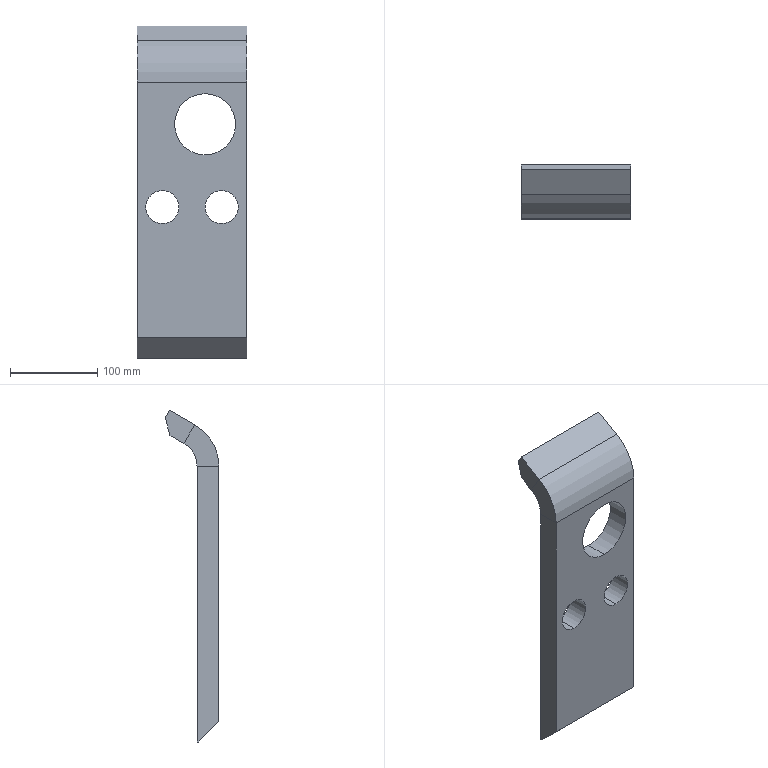Part | SolidWorks | features Chamfer 2, FlatPattern 1, ICE 1, SMBaseFlange 1, SheetMetal 1 | 1 solid | 22 faces | box 126 x 61.5 x 380.651 mm | volume 1041526 mm3 | plane 14 | cylinder 8 | commonest cylinder face diameters 38 x4 70 x2 60 x1 110 x1
STEP:
#1=CARTESIAN_POINT('',(15.,25.,130.));
#2=VERTEX_POINT('',#1);
#3=CARTESIAN_POINT('',(15.,25.,60.));
#4=VERTEX_POINT('',#3);
#5=CARTESIAN_POINT('',(15.,25.,95.));
#6=DIRECTION('',(0.,-1.,0.));
#7=DIRECTION('',(0.,0.,1.));
#8=AXIS2_PLACEMENT_3D('',#5,#6,#7);
#9=CIRCLE('',#8,35.);
#10=EDGE_CURVE('',#2,#4,#9,.T.);
#11=ORIENTED_EDGE('',*,*,#10,.F.);
#12=CARTESIAN_POINT('',(15.,0.,130.));
#13=VERTEX_POINT('',#12);
#14=CARTESIAN_POINT('',(15.,69.,130.));
#15=DIRECTION('',(0.,-1.,0.));
#16=VECTOR('',#15,1000.);
#17=LINE('',#14,#16);
#18=EDGE_CURVE('',#2,#13,#17,.T.);
#19=ORIENTED_EDGE('',*,*,#18,.T.);
#20=CARTESIAN_POINT('',(15.,0.,60.));
#21=VERTEX_POINT('',#20);
#22=CARTESIAN_POINT('',(15.,0.,95.));
#23=DIRECTION('',(0.,1.,0.));
#24=DIRECTION('',(0.,0.,1.));
#25=AXIS2_PLACEMENT_3D('',#22,#23,#24);
#26=CIRCLE('',#25,35.);
#27=EDGE_CURVE('',#21,#13,#26,.T.);
#28=ORIENTED_EDGE('',*,*,#27,.F.);
#29=CARTESIAN_POINT('',(15.,69.,60.));
#30=DIRECTION('',(0.,-1.,0.));
#31=VECTOR('',#30,1000.);
#32=LINE('',#29,#31);
#33=EDGE_CURVE('',#4,#21,#32,.T.);
#34=ORIENTED_EDGE('',*,*,#33,.F.);
#35=EDGE_LOOP('',(#11,#19,#28,#34));
#36=FACE_OUTER_BOUND('',#35,.T.);
#37=CARTESIAN_POINT('',(15.,69.,95.));
#38=DIRECTION('',(0.,-1.,0.));
#39=DIRECTION('',(0.,0.,-1.));
#40=AXIS2_PLACEMENT_3D('',#37,#38,#39);
#41=CYLINDRICAL_SURFACE('',#40,35.);
#42=ADVANCED_FACE('',(#36),#41,.F.);
#43=CARTESIAN_POINT('',(-34.,25.,19.));
#44=VERTEX_POINT('',#43);
#45=CARTESIAN_POINT('',(-34.,25.,-19.));
#46=VERTEX_POINT('',#45);
#47=CARTESIAN_POINT('',(-34.,25.,0.));
#48=DIRECTION('',(0.,-1.,0.));
#49=DIRECTION('',(0.,0.,1.));
#50=AXIS2_PLACEMENT_3D('',#47,#48,#49);
#51=CIRCLE('',#50,19.);
#52=EDGE_CURVE('',#44,#46,#51,.T.);
#53=ORIENTED_EDGE('',*,*,#52,.F.);
#54=CARTESIAN_POINT('',(-34.,0.,19.));
#55=VERTEX_POINT('',#54);
#56=CARTESIAN_POINT('',(-34.,69.,19.));
#57=DIRECTION('',(0.,-1.,0.));
#58=VECTOR('',#57,1000.);
#59=LINE('',#56,#58);
#60=EDGE_CURVE('',#44,#55,#59,.T.);
#61=ORIENTED_EDGE('',*,*,#60,.T.);
#62=CARTESIAN_POINT('',(-34.,0.,-19.));
#63=VERTEX_POINT('',#62);
#64=CARTESIAN_POINT('',(-34.,0.,0.));
#65=DIRECTION('',(0.,1.,0.));
#66=DIRECTION('',(0.,0.,1.));
#67=AXIS2_PLACEMENT_3D('',#64,#65,#66);
#68=CIRCLE('',#67,19.);
#69=EDGE_CURVE('',#63,#55,#68,.T.);
#70=ORIENTED_EDGE('',*,*,#69,.F.);
#71=CARTESIAN_POINT('',(-34.,69.,-19.));
#72=DIRECTION('',(0.,-1.,0.));
#73=VECTOR('',#72,1000.);
#74=LINE('',#71,#73);
#75=EDGE_CURVE('',#46,#63,#74,.T.);
#76=ORIENTED_EDGE('',*,*,#75,.F.);
#77=EDGE_LOOP('',(#53,#61,#70,#76));
#78=FACE_OUTER_BOUND('',#77,.T.);
#79=CARTESIAN_POINT('',(-34.,69.,0.));
#80=DIRECTION('',(0.,-1.,0.));
#81=DIRECTION('',(0.,0.,-1.));
#82=AXIS2_PLACEMENT_3D('',#79,#80,#81);
#83=CYLINDRICAL_SURFACE('',#82,19.);
#84=ADVANCED_FACE('',(#78),#83,.F.);
#85=CARTESIAN_POINT('',(34.,25.,19.));
#86=VERTEX_POINT('',#85);
#87=CARTESIAN_POINT('',(34.,25.,-19.));
#88=VERTEX_POINT('',#87);
#89=CARTESIAN_POINT('',(34.,25.,0.));
#90=DIRECTION('',(0.,-1.,0.));
#91=DIRECTION('',(0.,0.,1.));
#92=AXIS2_PLACEMENT_3D('',#89,#90,#91);
#93=CIRCLE('',#92,19.);
#94=EDGE_CURVE('',#86,#88,#93,.T.);
#95=ORIENTED_EDGE('',*,*,#94,.F.);
#96=CARTESIAN_POINT('',(34.,0.,19.));
#97=VERTEX_POINT('',#96);
#98=CARTESIAN_POINT('',(34.,69.,19.));
#99=DIRECTION('',(0.,-1.,0.));
#100=VECTOR('',#99,1000.);
#101=LINE('',#98,#100);
#102=EDGE_CURVE('',#86,#97,#101,.T.);
#103=ORIENTED_EDGE('',*,*,#102,.T.);
#104=CARTESIAN_POINT('',(34.,0.,-19.));
#105=VERTEX_POINT('',#104);
#106=CARTESIAN_POINT('',(34.,0.,0.));
#107=DIRECTION('',(0.,1.,0.));
#108=DIRECTION('',(0.,0.,1.));
#109=AXIS2_PLACEMENT_3D('',#106,#107,#108);
#110=CIRCLE('',#109,19.);
#111=EDGE_CURVE('',#105,#97,#110,.T.);
#112=ORIENTED_EDGE('',*,*,#111,.F.);
#113=CARTESIAN_POINT('',(34.,69.,-19.));
#114=DIRECTION('',(0.,-1.,0.));
#115=VECTOR('',#114,1000.);
#116=LINE('',#113,#115);
#117=EDGE_CURVE('',#88,#105,#116,.T.);
#118=ORIENTED_EDGE('',*,*,#117,.F.);
#119=EDGE_LOOP('',(#95,#103,#112,#118));
#120=FACE_OUTER_BOUND('',#119,.T.);
#121=CARTESIAN_POINT('',(34.,69.,0.));
#122=DIRECTION('',(0.,-1.,0.));
#123=DIRECTION('',(0.,0.,-1.));
#124=AXIS2_PLACEMENT_3D('',#121,#122,#123);
#125=CYLINDRICAL_SURFACE('',#124,19.);
#126=ADVANCED_FACE('',(#120),#125,.F.);
#127=ORIENTED_EDGE('',*,*,#69,.T.);
#128=CARTESIAN_POINT('',(-34.,0.,0.));
#129=DIRECTION('',(0.,1.,0.));
#130=DIRECTION('',(0.,0.,1.));
#131=AXIS2_PLACEMENT_3D('',#128,#129,#130);
#132=CIRCLE('',#131,19.);
#133=EDGE_CURVE('',#55,#63,#132,.T.);
#134=ORIENTED_EDGE('',*,*,#133,.T.);
#135=EDGE_LOOP('',(#127,#134));
#136=FACE_BOUND('',#135,.T.);
#137=CARTESIAN_POINT('',(-63.,0.,143.276));
#138=VERTEX_POINT('',#137);
#139=CARTESIAN_POINT('',(-63.,0.,-150.));
#140=VERTEX_POINT('',#139);
#141=CARTESIAN_POINT('',(-63.,0.,160.597));
#142=DIRECTION('',(0.,0.,-1.));
#143=VECTOR('',#142,1000.);
#144=LINE('',#141,#143);
#145=EDGE_CURVE('',#138,#140,#144,.T.);
#146=ORIENTED_EDGE('',*,*,#145,.T.);
#147=CARTESIAN_POINT('',(63.,0.,-150.));
#148=VERTEX_POINT('',#147);
#149=CARTESIAN_POINT('',(63.,0.,-150.));
#150=DIRECTION('',(1.,0.,0.));
#151=VECTOR('',#150,1000.);
#152=LINE('',#149,#151);
#153=EDGE_CURVE('',#140,#148,#152,.T.);
#154=ORIENTED_EDGE('',*,*,#153,.T.);
#155=CARTESIAN_POINT('',(63.,0.,143.276));
#156=VERTEX_POINT('',#155);
#157=CARTESIAN_POINT('',(63.,0.,160.597));
#158=DIRECTION('',(0.,0.,-1.));
#159=VECTOR('',#158,1000.);
#160=LINE('',#157,#159);
#161=EDGE_CURVE('',#156,#148,#160,.T.);
#162=ORIENTED_EDGE('',*,*,#161,.F.);
#163=CARTESIAN_POINT('',(63.,0.,143.276));
#164=DIRECTION('',(-1.,0.,0.));
#165=VECTOR('',#164,1000.);
#166=LINE('',#163,#165);
#167=EDGE_CURVE('',#156,#138,#166,.T.);
#168=ORIENTED_EDGE('',*,*,#167,.T.);
#169=EDGE_LOOP('',(#146,#154,#162,#168));
#170=FACE_OUTER_BOUND('',#169,.T.);
#171=ORIENTED_EDGE('',*,*,#111,.T.);
#172=CARTESIAN_POINT('',(34.,0.,0.));
#173=DIRECTION('',(0.,1.,0.));
#174=DIRECTION('',(0.,0.,1.));
#175=AXIS2_PLACEMENT_3D('',#172,#173,#174);
#176=CIRCLE('',#175,19.);
#177=EDGE_CURVE('',#97,#105,#176,.T.);
#178=ORIENTED_EDGE('',*,*,#177,.T.);
#179=EDGE_LOOP('',(#171,#178));
#180=FACE_BOUND('',#179,.T.);
#181=ORIENTED_EDGE('',*,*,#27,.T.);
#182=CARTESIAN_POINT('',(15.,0.,95.));
#183=DIRECTION('',(0.,1.,0.));
#184=DIRECTION('',(0.,0.,1.));
#185=AXIS2_PLACEMENT_3D('',#182,#183,#184);
#186=CIRCLE('',#185,35.);
#187=EDGE_CURVE('',#13,#21,#186,.T.);
#188=ORIENTED_EDGE('',*,*,#187,.T.);
#189=EDGE_LOOP('',(#181,#188));
#190=FACE_BOUND('',#189,.T.);
#191=CARTESIAN_POINT('',(63.,0.,160.597));
#192=DIRECTION('',(0.,1.,0.));
#193=DIRECTION('',(0.,0.,1.));
#194=AXIS2_PLACEMENT_3D('',#191,#192,#193);
#195=PLANE('',#194);
#196=ADVANCED_FACE('',(#136,#170,#180,#190),#195,.F.);
#197=CARTESIAN_POINT('',(-34.,25.,0.));
#198=DIRECTION('',(0.,-1.,0.));
#199=DIRECTION('',(0.,0.,1.));
#200=AXIS2_PLACEMENT_3D('',#197,#198,#199);
#201=CIRCLE('',#200,19.);
#202=EDGE_CURVE('',#46,#44,#201,.T.);
#203=ORIENTED_EDGE('',*,*,#202,.T.);
#204=ORIENTED_EDGE('',*,*,#52,.T.);
#205=EDGE_LOOP('',(#203,#204));
#206=FACE_BOUND('',#205,.T.);
#207=CARTESIAN_POINT('',(-63.,25.,143.276));
#208=VERTEX_POINT('',#207);
#209=CARTESIAN_POINT('',(-63.,25.,-173.));
#210=VERTEX_POINT('',#209);
#211=CARTESIAN_POINT('',(-63.,25.,160.597));
#212=DIRECTION('',(0.,0.,-1.));
#213=VECTOR('',#212,1000.);
#214=LINE('',#211,#213);
#215=EDGE_CURVE('',#208,#210,#214,.T.);
#216=ORIENTED_EDGE('',*,*,#215,.F.);
#217=CARTESIAN_POINT('',(63.,25.,143.276));
#218=VERTEX_POINT('',#217);
#219=CARTESIAN_POINT('',(63.,25.,143.276));
#220=DIRECTION('',(-1.,0.,0.));
#221=VECTOR('',#220,1000.);
#222=LINE('',#219,#221);
#223=EDGE_CURVE('',#218,#208,#222,.T.);
#224=ORIENTED_EDGE('',*,*,#223,.F.);
#225=CARTESIAN_POINT('',(63.,25.,-173.));
#226=VERTEX_POINT('',#225);
#227=CARTESIAN_POINT('',(63.,25.,160.597));
#228=DIRECTION('',(0.,0.,-1.));
#229=VECTOR('',#228,1000.);
#230=LINE('',#227,#229);
#231=EDGE_CURVE('',#218,#226,#230,.T.);
#232=ORIENTED_EDGE('',*,*,#231,.T.);
#233=CARTESIAN_POINT('',(63.,25.,-173.));
#234=DIRECTION('',(-1.,0.,0.));
#235=VECTOR('',#234,1000.);
#236=LINE('',#233,#235);
#237=EDGE_CURVE('',#226,#210,#236,.T.);
#238=ORIENTED_EDGE('',*,*,#237,.T.);
#239=EDGE_LOOP('',(#216,#224,#232,#238));
#240=FACE_OUTER_BOUND('',#239,.T.);
#241=CARTESIAN_POINT('',(34.,25.,0.));
#242=DIRECTION('',(0.,-1.,0.));
#243=DIRECTION('',(0.,0.,1.));
#244=AXIS2_PLACEMENT_3D('',#241,#242,#243);
#245=CIRCLE('',#244,19.);
#246=EDGE_CURVE('',#88,#86,#245,.T.);
#247=ORIENTED_EDGE('',*,*,#246,.T.);
#248=ORIENTED_EDGE('',*,*,#94,.T.);
#249=EDGE_LOOP('',(#247,#248));
#250=FACE_BOUND('',#249,.T.);
#251=CARTESIAN_POINT('',(15.,25.,95.));
#252=DIRECTION('',(0.,-1.,0.));
#253=DIRECTION('',(0.,0.,1.));
#254=AXIS2_PLACEMENT_3D('',#251,#252,#253);
#255=CIRCLE('',#254,35.);
#256=EDGE_CURVE('',#4,#2,#255,.T.);
#257=ORIENTED_EDGE('',*,*,#256,.T.);
#258=ORIENTED_EDGE('',*,*,#10,.T.);
#259=EDGE_LOOP('',(#257,#258));
#260=FACE_BOUND('',#259,.T.);
#261=CARTESIAN_POINT('',(63.,25.,160.597));
#262=DIRECTION('',(0.,1.,0.));
#263=DIRECTION('',(0.,0.,1.));
#264=AXIS2_PLACEMENT_3D('',#261,#262,#263);
#265=PLANE('',#264);
#266=ADVANCED_FACE('',(#206,#240,#250,#260),#265,.T.);
#267=CARTESIAN_POINT('',(63.,25.,143.276));
#268=DIRECTION('',(0.,-1.,0.));
#269=VECTOR('',#268,1000.);
#270=LINE('',#267,#269);
#271=EDGE_CURVE('',#218,#156,#270,.T.);
#272=ORIENTED_EDGE('',*,*,#271,.F.);
#273=CARTESIAN_POINT('',(63.,40.,169.257));
#274=VERTEX_POINT('',#273);
#275=CARTESIAN_POINT('',(63.,55.,143.276));
#276=DIRECTION('',(1.,0.,0.));
#277=DIRECTION('',(0.,0.,-1.));
#278=AXIS2_PLACEMENT_3D('',#275,#276,#277);
#279=CIRCLE('',#278,30.);
#280=EDGE_CURVE('',#274,#218,#279,.T.);
#281=ORIENTED_EDGE('',*,*,#280,.F.);
#282=CARTESIAN_POINT('',(63.,27.5,190.907));
#283=VERTEX_POINT('',#282);
#284=CARTESIAN_POINT('',(63.,27.5,190.907));
#285=DIRECTION('',(0.,0.5,-0.866));
#286=VECTOR('',#285,1000.);
#287=LINE('',#284,#286);
#288=EDGE_CURVE('',#283,#274,#287,.T.);
#289=ORIENTED_EDGE('',*,*,#288,.F.);
#290=CARTESIAN_POINT('',(63.,55.,143.276));
#291=DIRECTION('',(1.,0.,0.));
#292=DIRECTION('',(0.,0.,-1.));
#293=AXIS2_PLACEMENT_3D('',#290,#291,#292);
#294=CIRCLE('',#293,55.);
#295=EDGE_CURVE('',#283,#156,#294,.T.);
#296=ORIENTED_EDGE('',*,*,#295,.T.);
#297=EDGE_LOOP('',(#272,#281,#289,#296));
#298=FACE_OUTER_BOUND('',#297,.T.);
#299=CARTESIAN_POINT('',(63.,25.,143.276));
#300=DIRECTION('',(1.,0.,0.));
#301=DIRECTION('',(0.,0.,-1.));
#302=AXIS2_PLACEMENT_3D('',#299,#300,#301);
#303=PLANE('',#302);
#304=ADVANCED_FACE('',(#298),#303,.T.);
#305=ORIENTED_EDGE('',*,*,#161,.T.);
#306=CARTESIAN_POINT('',(63.,23.,-173.));
#307=VERTEX_POINT('',#306);
#308=CARTESIAN_POINT('',(63.,-156.704,6.704));
#309=DIRECTION('',(0.,0.7071,-0.7071));
#310=VECTOR('',#309,1000.);
#311=LINE('',#308,#310);
#312=EDGE_CURVE('',#148,#307,#311,.T.);
#313=ORIENTED_EDGE('',*,*,#312,.T.);
#314=CARTESIAN_POINT('',(63.,25.,-173.));
#315=DIRECTION('',(0.,-1.,0.));
#316=VECTOR('',#315,1000.);
#317=LINE('',#314,#316);
#318=EDGE_CURVE('',#226,#307,#317,.T.);
#319=ORIENTED_EDGE('',*,*,#318,.F.);
#320=ORIENTED_EDGE('',*,*,#231,.F.);
#321=ORIENTED_EDGE('',*,*,#271,.T.);
#322=EDGE_LOOP('',(#305,#313,#319,#320,#321));
#323=FACE_OUTER_BOUND('',#322,.T.);
#324=CARTESIAN_POINT('',(63.,27.5,190.907));
#325=DIRECTION('',(1.,0.,0.));
#326=DIRECTION('',(0.,0.,-1.));
#327=AXIS2_PLACEMENT_3D('',#324,#325,#326);
#328=PLANE('',#327);
#329=ADVANCED_FACE('',(#323),#328,.T.);
#330=CARTESIAN_POINT('',(-63.,40.,169.257));
#331=VERTEX_POINT('',#330);
#332=CARTESIAN_POINT('',(-63.,27.5,190.907));
#333=VERTEX_POINT('',#332);
#334=CARTESIAN_POINT('',(-63.,40.,169.257));
#335=DIRECTION('',(0.,-0.5,0.866));
#336=VECTOR('',#335,1000.);
#337=LINE('',#334,#336);
#338=EDGE_CURVE('',#331,#333,#337,.T.);
#339=ORIENTED_EDGE('',*,*,#338,.F.);
#340=CARTESIAN_POINT('',(-63.,55.,143.276));
#341=DIRECTION('',(1.,0.,0.));
#342=DIRECTION('',(0.,0.,-1.));
#343=AXIS2_PLACEMENT_3D('',#340,#341,#342);
#344=CIRCLE('',#343,30.);
#345=EDGE_CURVE('',#331,#208,#344,.T.);
#346=ORIENTED_EDGE('',*,*,#345,.T.);
#347=CARTESIAN_POINT('',(-63.,0.,143.276));
#348=DIRECTION('',(0.,1.,0.));
#349=VECTOR('',#348,1000.);
#350=LINE('',#347,#349);
#351=EDGE_CURVE('',#138,#208,#350,.T.);
#352=ORIENTED_EDGE('',*,*,#351,.F.);
#353=CARTESIAN_POINT('',(-63.,55.,143.276));
#354=DIRECTION('',(1.,0.,0.));
#355=DIRECTION('',(0.,0.,-1.));
#356=AXIS2_PLACEMENT_3D('',#353,#354,#355);
#357=CIRCLE('',#356,55.);
#358=EDGE_CURVE('',#333,#138,#357,.T.);
#359=ORIENTED_EDGE('',*,*,#358,.F.);
#360=EDGE_LOOP('',(#339,#346,#352,#359));
#361=FACE_OUTER_BOUND('',#360,.T.);
#362=CARTESIAN_POINT('',(-63.,40.,169.257));
#363=DIRECTION('',(-1.,0.,0.));
#364=DIRECTION('',(0.,0.,1.));
#365=AXIS2_PLACEMENT_3D('',#362,#363,#364);
#366=PLANE('',#365);
#367=ADVANCED_FACE('',(#361),#366,.T.);
#368=CARTESIAN_POINT('',(-63.,56.5,207.651));
#369=VERTEX_POINT('',#368);
#370=CARTESIAN_POINT('',(-63.,61.5,198.99));
#371=VERTEX_POINT('',#370);
#372=CARTESIAN_POINT('',(-63.,56.5,207.651));
#373=DIRECTION('',(0.,0.5,-0.866));
#374=VECTOR('',#373,1000.);
#375=LINE('',#372,#374);
#376=EDGE_CURVE('',#369,#371,#375,.T.);
#377=ORIENTED_EDGE('',*,*,#376,.T.);
#378=CARTESIAN_POINT('',(-63.,56.01,178.5));
#379=VERTEX_POINT('',#378);
#380=CARTESIAN_POINT('',(-63.,43.452,131.633));
#381=DIRECTION('',(0.,-0.2588,-0.9659));
#382=VECTOR('',#381,1000.);
#383=LINE('',#380,#382);
#384=EDGE_CURVE('',#371,#379,#383,.T.);
#385=ORIENTED_EDGE('',*,*,#384,.T.);
#386=CARTESIAN_POINT('',(-63.,25.,160.597));
#387=DIRECTION('',(0.,-0.866,-0.5));
#388=VECTOR('',#387,1000.);
#389=LINE('',#386,#388);
#390=EDGE_CURVE('',#379,#331,#389,.T.);
#391=ORIENTED_EDGE('',*,*,#390,.T.);
#392=ORIENTED_EDGE('',*,*,#338,.T.);
#393=CARTESIAN_POINT('',(-63.,12.5,182.247));
#394=DIRECTION('',(0.,-0.866,-0.5));
#395=VECTOR('',#394,1000.);
#396=LINE('',#393,#395);
#397=EDGE_CURVE('',#369,#333,#396,.T.);
#398=ORIENTED_EDGE('',*,*,#397,.F.);
#399=EDGE_LOOP('',(#377,#385,#391,#392,#398));
#400=FACE_OUTER_BOUND('',#399,.T.);
#401=CARTESIAN_POINT('',(-63.,0.,143.276));
#402=DIRECTION('',(-1.,0.,0.));
#403=DIRECTION('',(0.,0.,1.));
#404=AXIS2_PLACEMENT_3D('',#401,#402,#403);
#405=PLANE('',#404);
#406=ADVANCED_FACE('',(#400),#405,.T.);
#407=ORIENTED_EDGE('',*,*,#318,.T.);
#408=CARTESIAN_POINT('',(-63.,23.,-173.));
#409=VERTEX_POINT('',#408);
#410=CARTESIAN_POINT('',(-63.,23.,-173.));
#411=DIRECTION('',(-1.,0.,0.));
#412=VECTOR('',#411,1000.);
#413=LINE('',#410,#412);
#414=EDGE_CURVE('',#307,#409,#413,.T.);
#415=ORIENTED_EDGE('',*,*,#414,.T.);
#416=CARTESIAN_POINT('',(-63.,25.,-173.));
#417=DIRECTION('',(0.,-1.,0.));
#418=VECTOR('',#417,1000.);
#419=LINE('',#416,#418);
#420=EDGE_CURVE('',#210,#409,#419,.T.);
#421=ORIENTED_EDGE('',*,*,#420,.F.);
#422=ORIENTED_EDGE('',*,*,#237,.F.);
#423=EDGE_LOOP('',(#407,#415,#421,#422));
#424=FACE_OUTER_BOUND('',#423,.T.);
#425=CARTESIAN_POINT('',(63.,25.,-173.));
#426=DIRECTION('',(0.,0.,-1.));
#427=DIRECTION('',(0.,1.,0.));
#428=AXIS2_PLACEMENT_3D('',#425,#426,#427);
#429=PLANE('',#428);
#430=ADVANCED_FACE('',(#424),#429,.T.);
#431=ORIENTED_EDGE('',*,*,#345,.F.);
#432=CARTESIAN_POINT('',(63.,40.,169.257));
#433=DIRECTION('',(-1.,0.,0.));
#434=VECTOR('',#433,1000.);
#435=LINE('',#432,#434);
#436=EDGE_CURVE('',#274,#331,#435,.T.);
#437=ORIENTED_EDGE('',*,*,#436,.F.);
#438=ORIENTED_EDGE('',*,*,#280,.T.);
#439=ORIENTED_EDGE('',*,*,#223,.T.);
#440=EDGE_LOOP('',(#431,#437,#438,#439));
#441=FACE_OUTER_BOUND('',#440,.T.);
#442=CARTESIAN_POINT('',(63.,55.,143.276));
#443=DIRECTION('',(-1.,0.,0.));
#444=DIRECTION('',(0.,0.,1.));
#445=AXIS2_PLACEMENT_3D('',#442,#443,#444);
#446=CYLINDRICAL_SURFACE('',#445,30.);
#447=ADVANCED_FACE('',(#441),#446,.F.);
#448=ORIENTED_EDGE('',*,*,#390,.F.);
#449=CARTESIAN_POINT('',(63.,56.01,178.5));
#450=VERTEX_POINT('',#449);
#451=CARTESIAN_POINT('',(63.,56.01,178.5));
#452=DIRECTION('',(1.,0.,0.));
#453=VECTOR('',#452,1000.);
#454=LINE('',#451,#453);
#455=EDGE_CURVE('',#379,#450,#454,.T.);
#456=ORIENTED_EDGE('',*,*,#455,.T.);
#457=CARTESIAN_POINT('',(63.,25.,160.597));
#458=DIRECTION('',(0.,-0.866,-0.5));
#459=VECTOR('',#458,1000.);
#460=LINE('',#457,#459);
#461=EDGE_CURVE('',#450,#274,#460,.T.);
#462=ORIENTED_EDGE('',*,*,#461,.T.);
#463=ORIENTED_EDGE('',*,*,#436,.T.);
#464=EDGE_LOOP('',(#448,#456,#462,#463));
#465=FACE_OUTER_BOUND('',#464,.T.);
#466=CARTESIAN_POINT('',(63.,25.,160.597));
#467=DIRECTION('',(0.,0.5,-0.866));
#468=DIRECTION('',(0.,0.866,0.5));
#469=AXIS2_PLACEMENT_3D('',#466,#467,#468);
#470=PLANE('',#469);
#471=ADVANCED_FACE('',(#465),#470,.T.);
#472=CARTESIAN_POINT('',(63.,56.5,207.651));
#473=VERTEX_POINT('',#472);
#474=CARTESIAN_POINT('',(63.,61.5,198.99));
#475=VERTEX_POINT('',#474);
#476=CARTESIAN_POINT('',(63.,56.5,207.651));
#477=DIRECTION('',(0.,0.5,-0.866));
#478=VECTOR('',#477,1000.);
#479=LINE('',#476,#478);
#480=EDGE_CURVE('',#473,#475,#479,.T.);
#481=ORIENTED_EDGE('',*,*,#480,.T.);
#482=CARTESIAN_POINT('',(63.,61.5,198.99));
#483=DIRECTION('',(-1.,0.,0.));
#484=VECTOR('',#483,1000.);
#485=LINE('',#482,#484);
#486=EDGE_CURVE('',#475,#371,#485,.T.);
#487=ORIENTED_EDGE('',*,*,#486,.T.);
#488=ORIENTED_EDGE('',*,*,#376,.F.);
#489=CARTESIAN_POINT('',(63.,56.5,207.651));
#490=DIRECTION('',(-1.,0.,0.));
#491=VECTOR('',#490,1000.);
#492=LINE('',#489,#491);
#493=EDGE_CURVE('',#473,#369,#492,.T.);
#494=ORIENTED_EDGE('',*,*,#493,.F.);
#495=EDGE_LOOP('',(#481,#487,#488,#494));
#496=FACE_OUTER_BOUND('',#495,.T.);
#497=CARTESIAN_POINT('',(63.,56.5,207.651));
#498=DIRECTION('',(0.,0.866,0.5));
#499=DIRECTION('',(0.,-0.5,0.866));
#500=AXIS2_PLACEMENT_3D('',#497,#498,#499);
#501=PLANE('',#500);
#502=ADVANCED_FACE('',(#496),#501,.T.);
#503=ORIENTED_EDGE('',*,*,#397,.T.);
#504=CARTESIAN_POINT('',(63.,27.5,190.907));
#505=DIRECTION('',(-1.,0.,0.));
#506=VECTOR('',#505,1000.);
#507=LINE('',#504,#506);
#508=EDGE_CURVE('',#283,#333,#507,.T.);
#509=ORIENTED_EDGE('',*,*,#508,.F.);
#510=CARTESIAN_POINT('',(63.,12.5,182.247));
#511=DIRECTION('',(0.,-0.866,-0.5));
#512=VECTOR('',#511,1000.);
#513=LINE('',#510,#512);
#514=EDGE_CURVE('',#473,#283,#513,.T.);
#515=ORIENTED_EDGE('',*,*,#514,.F.);
#516=ORIENTED_EDGE('',*,*,#493,.T.);
#517=EDGE_LOOP('',(#503,#509,#515,#516));
#518=FACE_OUTER_BOUND('',#517,.T.);
#519=CARTESIAN_POINT('',(63.,12.5,182.247));
#520=DIRECTION('',(0.,0.5,-0.866));
#521=DIRECTION('',(0.,0.866,0.5));
#522=AXIS2_PLACEMENT_3D('',#519,#520,#521);
#523=PLANE('',#522);
#524=ADVANCED_FACE('',(#518),#523,.F.);
#525=ORIENTED_EDGE('',*,*,#358,.T.);
#526=ORIENTED_EDGE('',*,*,#167,.F.);
#527=ORIENTED_EDGE('',*,*,#295,.F.);
#528=ORIENTED_EDGE('',*,*,#508,.T.);
#529=EDGE_LOOP('',(#525,#526,#527,#528));
#530=FACE_OUTER_BOUND('',#529,.T.);
#531=CARTESIAN_POINT('',(63.,55.,143.276));
#532=DIRECTION('',(-1.,0.,0.));
#533=DIRECTION('',(0.,0.,1.));
#534=AXIS2_PLACEMENT_3D('',#531,#532,#533);
#535=CYLINDRICAL_SURFACE('',#534,55.);
#536=ADVANCED_FACE('',(#530),#535,.T.);
#537=ORIENTED_EDGE('',*,*,#461,.F.);
#538=CARTESIAN_POINT('',(63.,47.136,145.383));
#539=DIRECTION('',(0.,0.2588,0.9659));
#540=VECTOR('',#539,1000.);
#541=LINE('',#538,#540);
#542=EDGE_CURVE('',#450,#475,#541,.T.);
#543=ORIENTED_EDGE('',*,*,#542,.T.);
#544=ORIENTED_EDGE('',*,*,#480,.F.);
#545=ORIENTED_EDGE('',*,*,#514,.T.);
#546=ORIENTED_EDGE('',*,*,#288,.T.);
#547=EDGE_LOOP('',(#537,#543,#544,#545,#546));
#548=FACE_OUTER_BOUND('',#547,.T.);
#549=CARTESIAN_POINT('',(63.,55.,143.276));
#550=DIRECTION('',(1.,0.,0.));
#551=DIRECTION('',(0.,0.,-1.));
#552=AXIS2_PLACEMENT_3D('',#549,#550,#551);
#553=PLANE('',#552);
#554=ADVANCED_FACE('',(#548),#553,.T.);
#555=ORIENTED_EDGE('',*,*,#420,.T.);
#556=CARTESIAN_POINT('',(-63.,23.,-173.));
#557=DIRECTION('',(0.,-0.7071,0.7071));
#558=VECTOR('',#557,1000.);
#559=LINE('',#556,#558);
#560=EDGE_CURVE('',#409,#140,#559,.T.);
#561=ORIENTED_EDGE('',*,*,#560,.T.);
#562=ORIENTED_EDGE('',*,*,#145,.F.);
#563=ORIENTED_EDGE('',*,*,#351,.T.);
#564=ORIENTED_EDGE('',*,*,#215,.T.);
#565=EDGE_LOOP('',(#555,#561,#562,#563,#564));
#566=FACE_OUTER_BOUND('',#565,.T.);
#567=CARTESIAN_POINT('',(-63.,55.,143.276));
#568=DIRECTION('',(1.,0.,0.));
#569=DIRECTION('',(0.,0.,-1.));
#570=AXIS2_PLACEMENT_3D('',#567,#568,#569);
#571=PLANE('',#570);
#572=ADVANCED_FACE('',(#566),#571,.F.);
#573=ORIENTED_EDGE('',*,*,#102,.F.);
#574=ORIENTED_EDGE('',*,*,#246,.F.);
#575=ORIENTED_EDGE('',*,*,#117,.T.);
#576=ORIENTED_EDGE('',*,*,#177,.F.);
#577=EDGE_LOOP('',(#573,#574,#575,#576));
#578=FACE_OUTER_BOUND('',#577,.T.);
#579=CARTESIAN_POINT('',(34.,69.,0.));
#580=DIRECTION('',(0.,-1.,0.));
#581=DIRECTION('',(0.,0.,-1.));
#582=AXIS2_PLACEMENT_3D('',#579,#580,#581);
#583=CYLINDRICAL_SURFACE('',#582,19.);
#584=ADVANCED_FACE('',(#578),#583,.F.);
#585=ORIENTED_EDGE('',*,*,#60,.F.);
#586=ORIENTED_EDGE('',*,*,#202,.F.);
#587=ORIENTED_EDGE('',*,*,#75,.T.);
#588=ORIENTED_EDGE('',*,*,#133,.F.);
#589=EDGE_LOOP('',(#585,#586,#587,#588));
#590=FACE_OUTER_BOUND('',#589,.T.);
#591=CARTESIAN_POINT('',(-34.,69.,0.));
#592=DIRECTION('',(0.,-1.,0.));
#593=DIRECTION('',(0.,0.,-1.));
#594=AXIS2_PLACEMENT_3D('',#591,#592,#593);
#595=CYLINDRICAL_SURFACE('',#594,19.);
#596=ADVANCED_FACE('',(#590),#595,.F.);
#597=ORIENTED_EDGE('',*,*,#18,.F.);
#598=ORIENTED_EDGE('',*,*,#256,.F.);
#599=ORIENTED_EDGE('',*,*,#33,.T.);
#600=ORIENTED_EDGE('',*,*,#187,.F.);
#601=EDGE_LOOP('',(#597,#598,#599,#600));
#602=FACE_OUTER_BOUND('',#601,.T.);
#603=CARTESIAN_POINT('',(15.,69.,95.));
#604=DIRECTION('',(0.,-1.,0.));
#605=DIRECTION('',(0.,0.,-1.));
#606=AXIS2_PLACEMENT_3D('',#603,#604,#605);
#607=CYLINDRICAL_SURFACE('',#606,35.);
#608=ADVANCED_FACE('',(#602),#607,.F.);
#609=ORIENTED_EDGE('',*,*,#312,.F.);
#610=ORIENTED_EDGE('',*,*,#153,.F.);
#611=ORIENTED_EDGE('',*,*,#560,.F.);
#612=ORIENTED_EDGE('',*,*,#414,.F.);
#613=EDGE_LOOP('',(#609,#610,#611,#612));
#614=FACE_OUTER_BOUND('',#613,.T.);
#615=CARTESIAN_POINT('',(63.,23.,-173.));
#616=DIRECTION('',(0.,-0.7071,-0.7071));
#617=DIRECTION('',(1.,0.,0.));
#618=AXIS2_PLACEMENT_3D('',#615,#616,#617);
#619=PLANE('',#618);
#620=ADVANCED_FACE('',(#614),#619,.T.);
#621=ORIENTED_EDGE('',*,*,#542,.F.);
#622=ORIENTED_EDGE('',*,*,#455,.F.);
#623=ORIENTED_EDGE('',*,*,#384,.F.);
#624=ORIENTED_EDGE('',*,*,#486,.F.);
#625=EDGE_LOOP('',(#621,#622,#623,#624));
#626=FACE_OUTER_BOUND('',#625,.T.);
#627=CARTESIAN_POINT('',(63.,61.5,198.99));
#628=DIRECTION('',(0.,-0.9659,0.2588));
#629=DIRECTION('',(-1.,0.,0.));
#630=AXIS2_PLACEMENT_3D('',#627,#628,#629);
#631=PLANE('',#630);
#632=ADVANCED_FACE('',(#626),#631,.F.);
#633=CLOSED_SHELL('',(#42,#84,#126,#196,#266,#304,#329,#367,#406,#430,#447,#471,#502,#524,#536,#554,#572,#584,#596,#608,#620,#632));
#634=MANIFOLD_SOLID_BREP('',#633);
#635=CARTESIAN_POINT('',(0.,0.,0.));
#636=DIRECTION('',(0.,0.,1.));
#637=DIRECTION('',(1.,0.,0.));
#638=AXIS2_PLACEMENT_3D('',#635,#636,#637);
#639=(LENGTH_UNIT()NAMED_UNIT(*)SI_UNIT(.MILLI.,.METRE.));
#640=UNCERTAINTY_MEASURE_WITH_UNIT(LENGTH_MEASURE(0.00001),#639,'','');
#641=(NAMED_UNIT(*)PLANE_ANGLE_UNIT()SI_UNIT($,.RADIAN.));
#642=(NAMED_UNIT(*)SI_UNIT($,.STERADIAN.)SOLID_ANGLE_UNIT());
#643=(GEOMETRIC_REPRESENTATION_CONTEXT(3)GLOBAL_UNCERTAINTY_ASSIGNED_CONTEXT((#640))GLOBAL_UNIT_ASSIGNED_CONTEXT((#639,#641,#642))REPRESENTATION_CONTEXT('',''));
#644=ADVANCED_BREP_SHAPE_REPRESENTATION('',(#634,#638),#643);